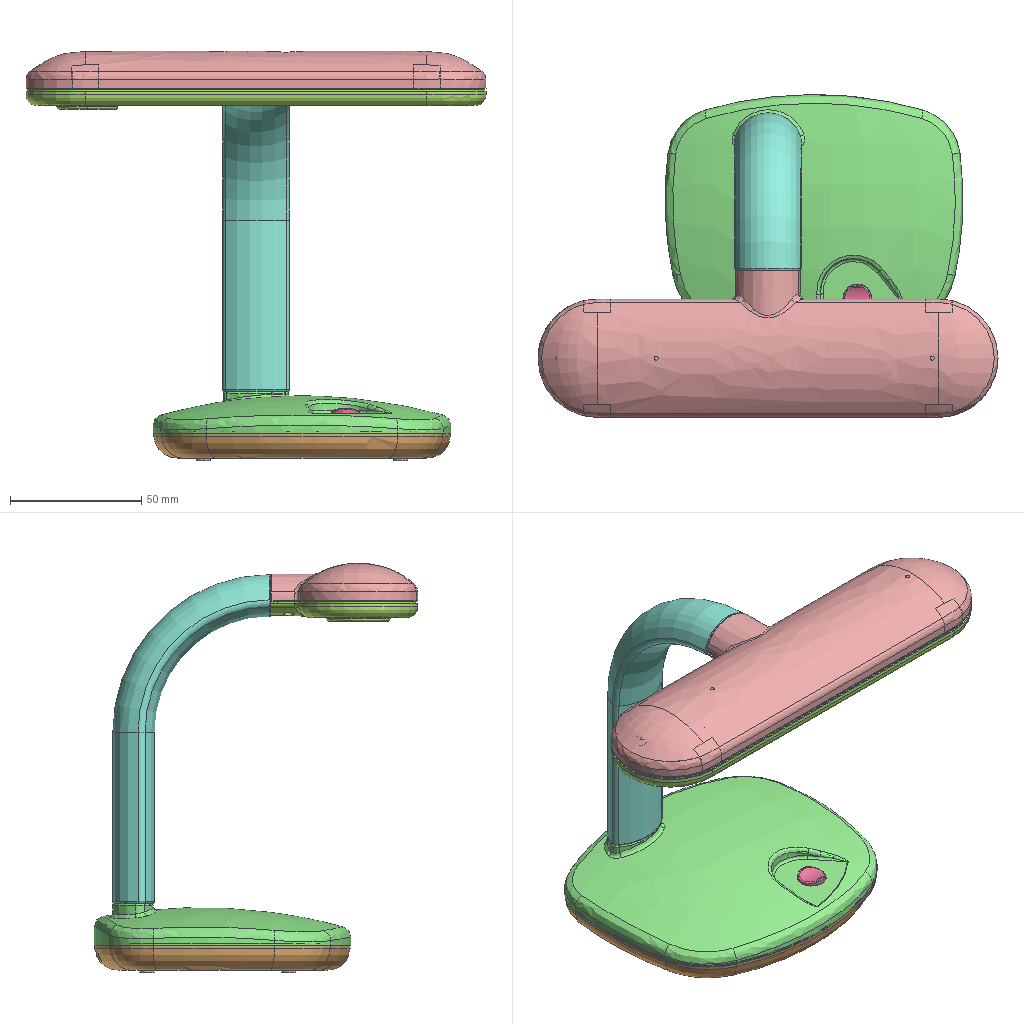Assembly | NX | 11 different items | 11 placed | box 175 x 123 x 156 mm
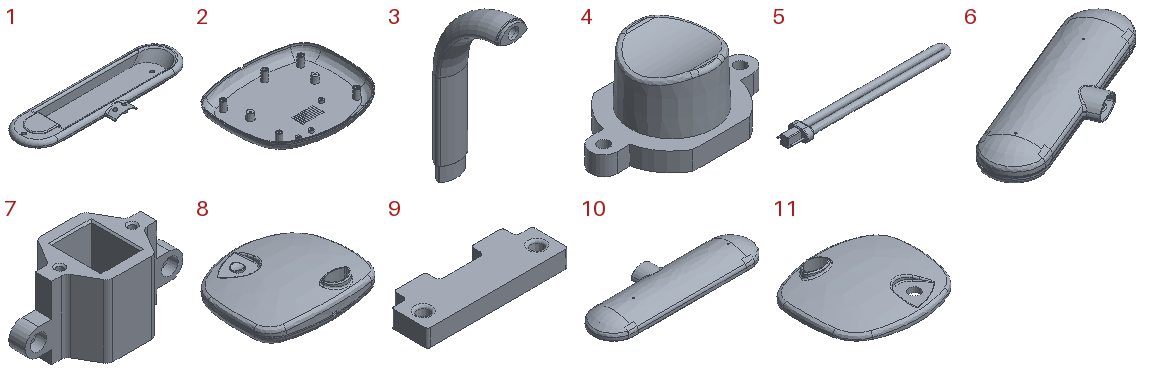Parts list (item | quantity | parent item | size | volume | features):
1 | x1 | in 6 | 175 x 56 x 16 mm | 12208 mm3 | features SKETCH 14, BLEND 8, EXTRUDE 8, CBORE_HOLE 5, DATUM_PLANE 3, HOLE PACKAGE 3, DATUM_CSYS 2, SCALE 2, SHELL 2, TRIM BODY 2, UNITE 2, CHAMFER 1, CPROJ 1, EXTRACT_FACE 1, SWP104 1, THRU_CURVE 1, TRIM_AND_EXTEND 1
2 | x1 | in 8 | 113.209 x 97.55 x 11.5 mm | 12367 mm3 | features EXTRACT_DATUM_PLANE 44, EXTRUDE 30, SKETCH 30, EXTRACT_DATUM_AXIS 22, Instance Feature 21, SIMPLE HOLE 5, CBORE_HOLE 4, DRAFT 4, HOLE PACKAGE 3, DATUM_CSYS 2, BLEND 1, Pattern Feature 1, SCALE 1, SHELL 1
3 | x1 | - | 25.275 x 62.5 x 137.498 mm | 37253 mm3 | features DATUM_CSYS 5, SKETCH 4, BLEND 2, EXTRUDE 2, SCALE 1, SWP104 1
4 | x1 | in 8 | 21.5 x 13 x 9.5 mm | 1029 mm3 | features DATUM_CSYS 4, EXTRUDE 3, SKETCH 3, BLEND 2, CBORE_HOLE 2, HOLE PACKAGE 2, DRAFT 1, SCALE 1
5 | x1 | in 6 | 131.993 x 16 x 9 mm | 5457 mm3 | features BLEND 7, DATUM_CSYS 7, SKETCH 6, EXTRUDE 4, SCALE 1, SKIN 1
6 | x1 | - | 165.085 x 94.798 x 22.148 mm | 29752 mm3 | features SKETCH 36, EXTRUDE 25, BLEND 21, DATUM_CSYS 15, HOLE PACKAGE 12, CBORE_HOLE 7, SIMPLE HOLE 7, DATUM_PLANE 6, SCALE 5, CHAMFER 3, EXTRACT_BODY 3, SEW 3, THRU_CURVE 3, THRU_CURVE_MESH 3, TRIM BODY 3, UNITE 3, BRIDGE_CURVE 2, CPROJ 2, Container 2, EXTRACT_FACE 2, Geometry Instance 2, SHELL 2, SWP104 2, TRIM_AND_EXTEND 2, DRAFT 1, SKIN 1, THICKEN_SHEET 1
7 | x1 | in 6 | 24 x 11 x 11 mm | 869.205 mm3 | features DATUM_CSYS 4, EXTRUDE 3, SKETCH 3, CBORE_HOLE 2, HOLE PACKAGE 2, BLEND 1, CHAMFER 1, SCALE 1
8 | x1 | - | 113.32 x 97.651 x 26.5 mm | 44372 mm3 | features SKETCH 49, EXTRUDE 45, EXTRACT_DATUM_PLANE 44, EXTRACT_DATUM_AXIS 22, Instance Feature 21, BLEND 13, SIMPLE HOLE 13, DATUM_CSYS 11, HOLE PACKAGE 9, DRAFT 8, CBORE_HOLE 6, TRIMMED_SH 6, SCALE 4, SEW 3, DATUM_PLANE 2, CHAMFER 1, Pattern Feature 1, SHELL 1, SKIN 1, THICKEN_SHEET 1
9 | x1 | in 8 | 77.5 x 27.5 x 10 mm | 17549 mm3 | features BLEND 3, DATUM_CSYS 3, EXTRUDE 2, SKETCH 2, CHAMFER 1, DRAFT 1, SCALE 1
10 | x1 | in 6 | 175 x 56.021 x 14.648 mm | 11136 mm3 | features SKETCH 13, EXTRUDE 10, HOLE PACKAGE 7, SIMPLE HOLE 7, BLEND 5, DATUM_PLANE 3, EXTRACT_BODY 3, SEW 3, THRU_CURVE_MESH 3, BRIDGE_CURVE 2, Container 2, DATUM_CSYS 2, Geometry Instance 2, THRU_CURVE 2, CHAMFER 1, CPROJ 1, DRAFT 1, EXTRACT_FACE 1, SCALE 1, SWP104 1, THICKEN_SHEET 1, TRIM BODY 1, TRIM_AND_EXTEND 1, UNITE 1
11 | x1 | in 8 | 113.32 x 97.651 x 16.5 mm | 13427 mm3 | features SKETCH 14, EXTRUDE 10, SIMPLE HOLE 8, BLEND 7, TRIMMED_SH 6, HOLE PACKAGE 4, SEW 3, DATUM_CSYS 2, DATUM_PLANE 2, DRAFT 2, SCALE 1, SKIN 1, THICKEN_SHEET 1
Mates (type | each side: item.copy, entity, surface, feature):
In the top assembly
Touch | 11.1 face plane Extrude(24) | 3.1 face plane Extrude(4)
Touch | 3.1 face cylinder Extrude(4) | 11.1 face cylinder Extrude(24)
Touch | 10.1 face plane Extrude(50) | 3.1 face plane Sweep(3)
Touch | 10.1 face cylinder Extrude(26) | 3.1 face cylinder Extrude(5)
Parallel | 1.1 face plane Extrude(3) | 2.1 face plane Extrude(1)
Fix | 8.1 component
In subassembly 6
Fix | 10.1 component
Distance | 10.1 | 1.1
In subassembly 8
Touch | 9.1 | 2.1 | 2 times
Touch | 11.1 | 2.1 | 3 times
Touch | 4.1 | 11.1 | 2 times
Touch | 11.1 | 4.1
Fix | 2.1 component
Distance | 11.1 | 2.1